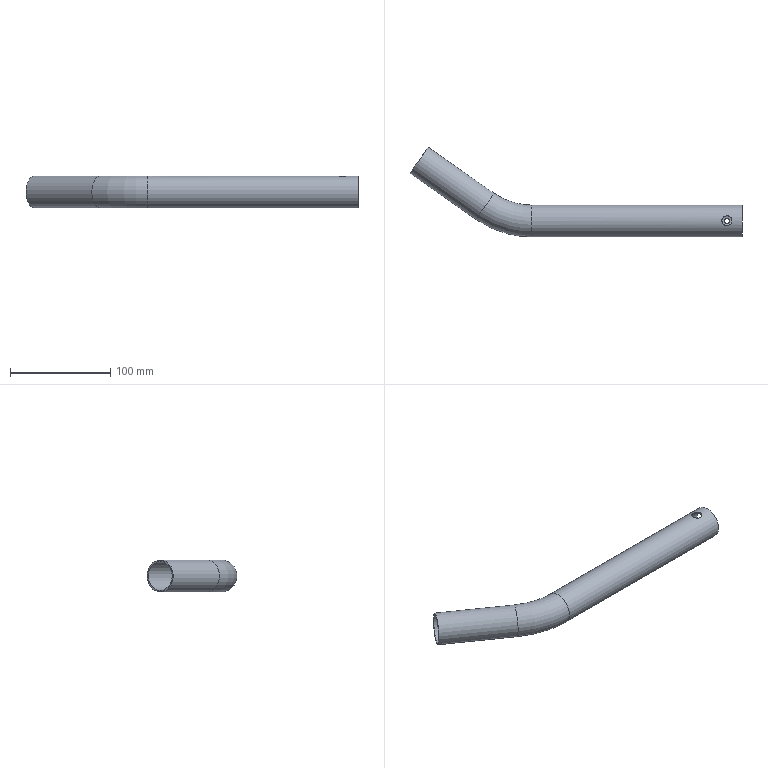Part | STEP file | Q7C1207L | 1 solid | 10 faces | box 330.538 x 89.278 x 31.8 mm | volume 48236 mm3 | cylinder 6 | torus 2 | plane 2 | commonest cylinder face diameters 28.8 x2 31.8 x2 5 x1 10 x1